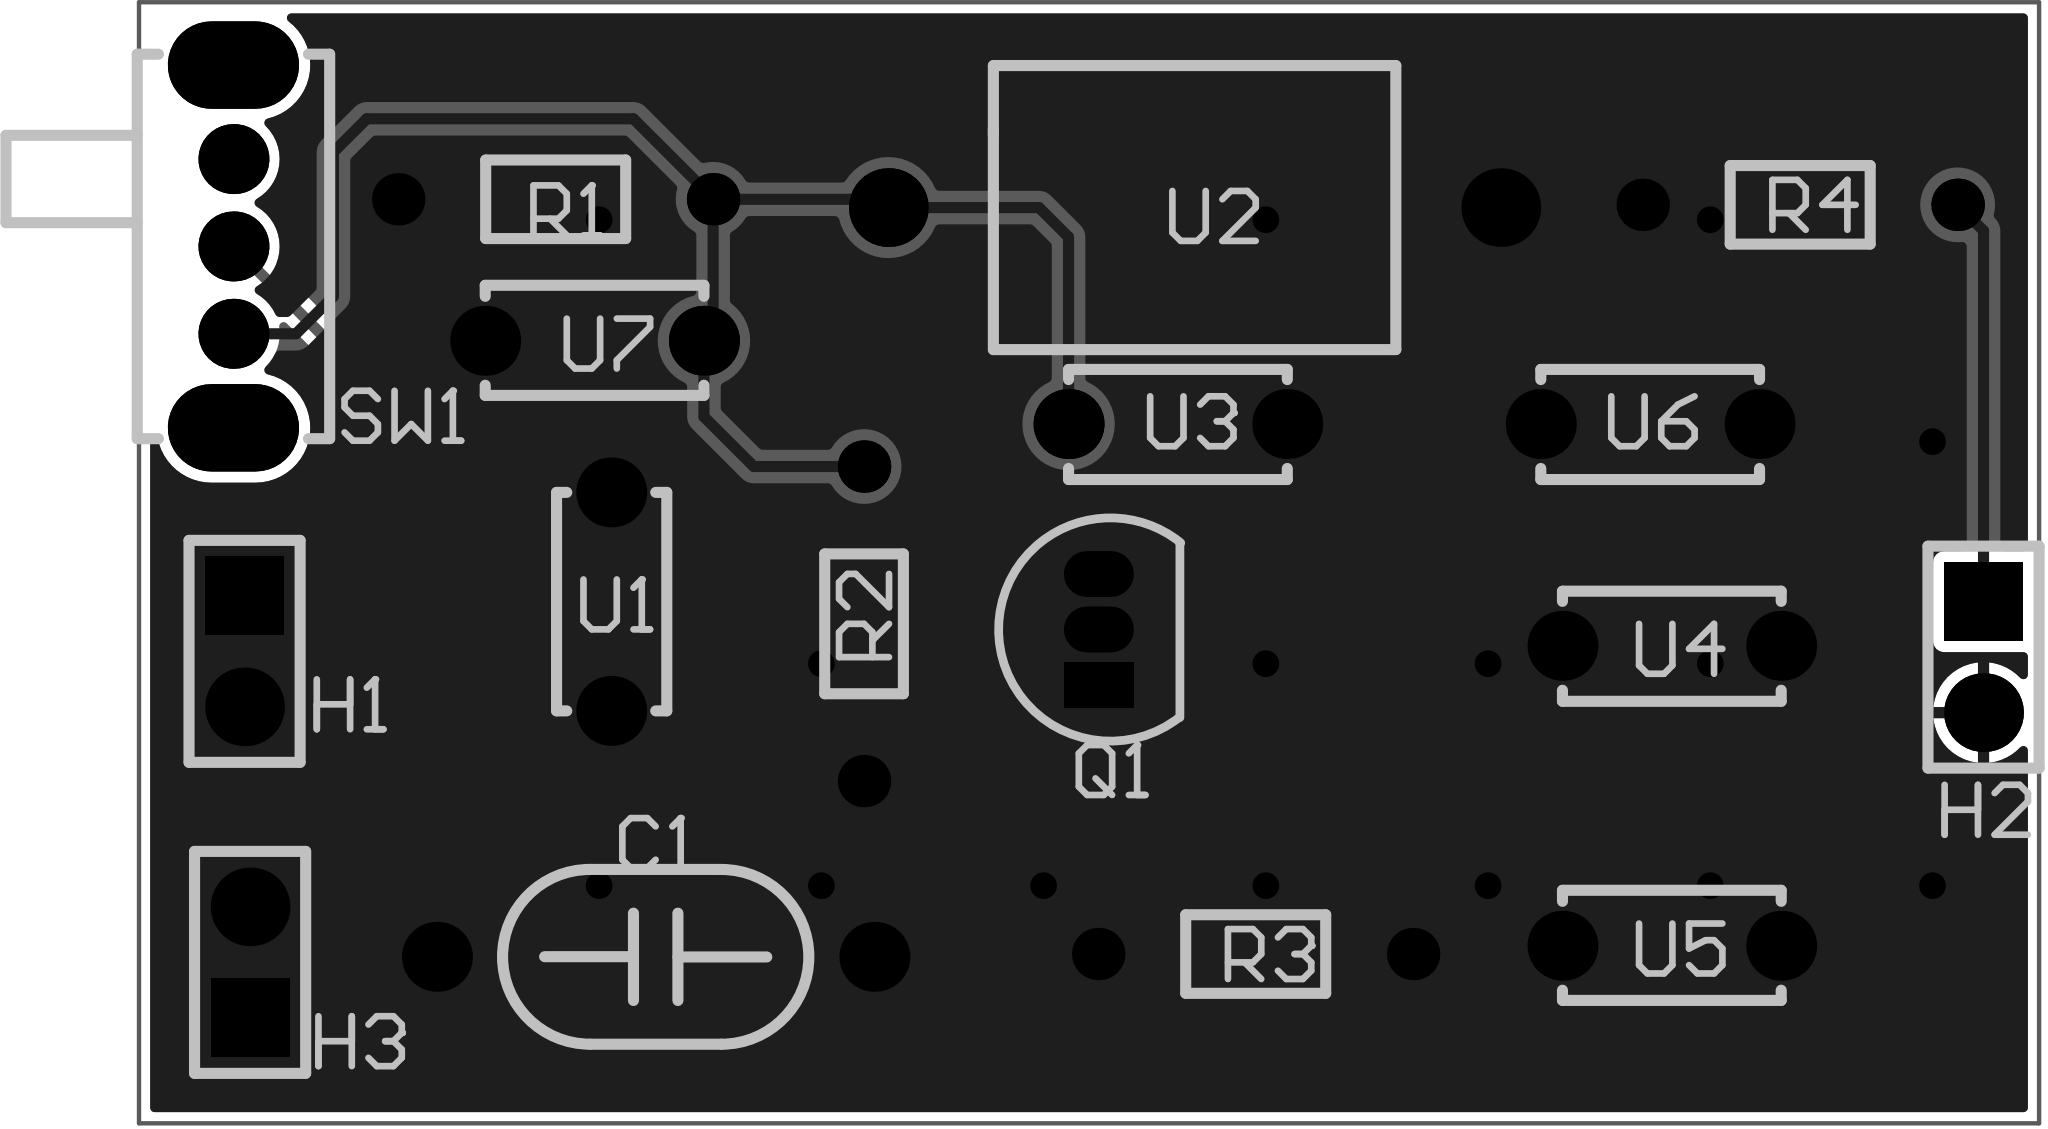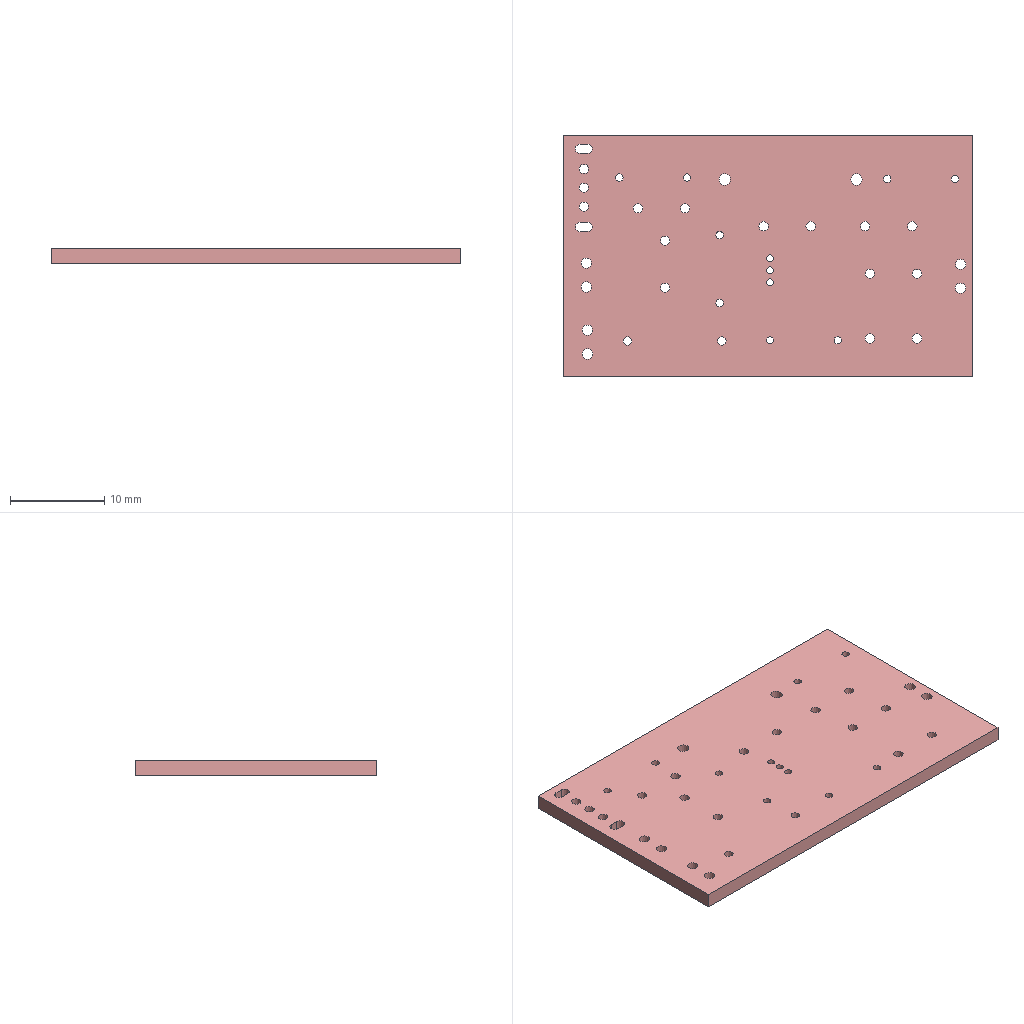Circuit board layout | Altium Designer | box 43.4 x 25.7 x 1.6 mm
Layer stack:
# Altium Designer layer stack of  (unit mm; dielectric type: 0 none, 1 core, 2 prepreg, 3 surface material)
index,name,kind,layer,copper_thickness_mm,dielectric_type,dielectric_thickness_mm,dielectric_material,dielectric_constant
0,Top Paste Mask Layer,other,,,,,,
1,Top Silkscreen Layer,other,,,,,,
2,Top Solder Mask Layer,dielectric,,,3,0.01,,3.3
3,Top Layer,copper,Top Layer,0.035,,,,
4,Dielectric1,dielectric,,,3,1.51,FR4,4.5
5,Bottom Layer,copper,Bottom Layer,0.035,,,,
6,Bottom Solder Mask Layer,dielectric,,,3,0.01,,3.3
7,Bottom Silkscreen Layer,other,,,,,,
8,Bottom Paste Mask Layer,other,,,,,,
# drill layer pairs: low layer,high layer
drill_pair,Top Layer,Bottom Layer
Part placement:
Designator,Comment,Layer,Footprint,Center-X(mm),Center-Y(mm),Rotation
C1,1nF,TopLayer,CAP-TH_L7.0-W4.0-P10.00-D0.6-1,91.239,87.376,0
H1,,TopLayer,HDR-TH_2P-P2.54-V-M-1,81.841,94.366,270
H2,,TopLayer,HDR-TH_2P-P2.54-V-M-1,121.592,94.234,270
H3,,TopLayer,HDR-TH_2P-P2.54-V-M-1,81.968,87.249,90
Q1,2N2222A,TopLayer,TO-92-3_L5.1-W4.1-P1.27-L-1,101.371,94.866,90
R1,2.2kΩ,TopLayer,Res_1/8W,88.953,104.711,0
R2,20kΩ,TopLayer,Res_1/8W,96.002,94.996,90
R3,220Ω,TopLayer,Res_1/8W,104.955,87.44,180
R4,50Ω,TopLayer,Res_1/8W,117.401,104.584,0
SW1,,TopLayer,拨动开关_侧,81.587,103.632,270
U1,100nF,TopLayer,CAP-TH_L5.0-W2.5-P5.00-D1.0,90.223,95.504,90
U2,0.08uH,TopLayer,IND-TH_BD6.5-W9.2-LS14.0-D0.8,103.558,104.521,0
U3,25pF,TopLayer,CAP-TH_L5.0-W2.5-P5.00-D1.0,103.177,99.568,0
U4,10pF,TopLayer,CAP-TH_L5.0-W2.5-P5.00-D1.0,114.467,94.493,0
U5,30pF,TopLayer,CAP-TH_L5.0-W2.5-P5.00-D1.0,114.468,87.629,180
U6,10pF,TopLayer,CAP-TH_L5.0-W2.5-P5.00-D1.0,113.972,99.568,0
U7,100nF,TopLayer,CAP-TH_L5.0-W2.5-P5.00-D1.0,89.843,101.473,180
Pad and via stacks:
# Altium Designer via and pad stacks of  (unit mm). Each distinct definition once, with the count of objects using it.
# via: kind,start_layer,end_layer,hole_mm,diameter_mm,mode(0 simple;1 top-mid-bottom;2 full stack),diameter_per_layer,count,example_net
# pad: kind,layer,hole_mm,hole_type(0 round;1 square;2 slot),plating,top_size,top_shape(1 round;2 rect;3 octagon;9 rounded rect),mid_size,bottom_size,mode,footprint,size_per_layer,count,example
pad,Multi-Layer,0.9144,0,plated,1.6x1.6,1,1.6x1.6,1.6x1.6,0,CAP-TH_L7.0-W4.0-P10.00-D0.6-1,,2,C1.1
pad,Multi-Layer,1.1,0,plated,1.8x1.8,1,1.8x1.8,1.8x1.8,0,HDR-TH_2P-P2.54-V-M-1,,3,H1.2
pad,Multi-Layer,1.1,0,plated,1.8x1.8,2,1.8x1.8,1.8x1.8,0,HDR-TH_2P-P2.54-V-M-1,,3,H1.1
pad,Multi-Layer,0.75,0,plated,1.05x1.6,2,1.05x1.6,1.05x1.6,0,TO-92-3_L5.1-W4.1-P1.27-L-1,,1,Q1.1
pad,Multi-Layer,0.75,0,plated,1.05x1.6,1,1.05x1.6,1.05x1.6,0,TO-92-3_L5.1-W4.1-P1.27-L-1,,2,Q1.2
pad,Multi-Layer,0.8001,0,plated,1.199x1.199,1,1.199x1.199,1.199x1.199,0,Res_1/8W,,8,R1.1
pad,Multi-Layer,1.001,0,plated,1.6x1.6,1,1.6x1.6,1.6x1.6,0,\u00B2\u00A6\u00B6\u00AF\u00BF\u00AA\u00B9\u00D8_\u00B2\u00E0,,3,SW1.1
pad,Multi-Layer,1.001,2,plated,3x1.999,1,3x1.999,3x1.999,0,\u00B2\u00A6\u00B6\u00AF\u00BF\u00AA\u00B9\u00D8_\u00B2\u00E0,,2,SW1.4
pad,Multi-Layer,1,0,plated,1.6x1.6,1,1.6x1.6,1.6x1.6,0,CAP-TH_L5.0-W2.5-P5.00-D1.0,,12,U1.1
pad,Multi-Layer,1.2,0,plated,1.8x1.8,1,1.8x1.8,1.8x1.8,0,IND-TH_BD6.5-W9.2-LS14.0-D0.8,,2,U2.1
via,Top Layer,Bottom Layer,0.3048,0.61,0,,15,GND
Copper pours:
name,layer,net,type(0 solid;1 hatched;2 none)
Top Layer-GND,Top Layer,GND,0
Bottom Layer-GND,Bottom Layer,GND,0